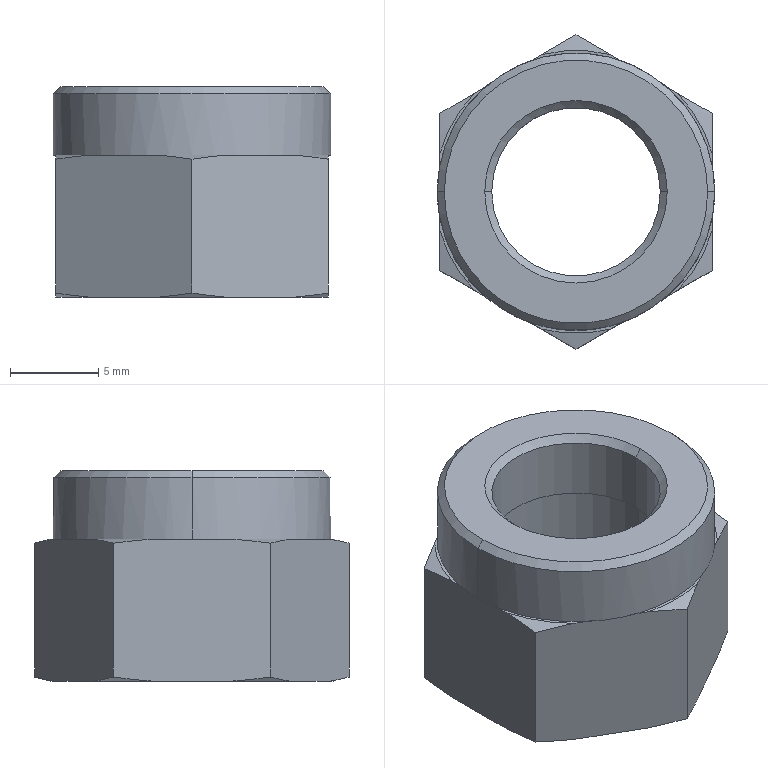Part | SolidWorks | features Cut 3, Boss 1, Chamfer 1, Extrusion 1 | 1 solid | 43 faces | box 15.68 x 17.77 x 11.9 mm | volume 1480 mm3 | plane 21 | cone 16 | cylinder 6 | commonest cylinder face diameters 9.524 x2 10 x2 15.68 x2
STEP:
#1=CARTESIAN_POINT('',(-4.762,0.,11.5));
#2=VERTEX_POINT('',#1);
#3=CARTESIAN_POINT('',(4.762,0.,11.5));
#4=VERTEX_POINT('',#3);
#5=CARTESIAN_POINT('',(0.,0.,11.5));
#6=DIRECTION('',(0.,0.,1.));
#7=DIRECTION('',(1.,0.,0.));
#8=AXIS2_PLACEMENT_3D('',#5,#6,#7);
#9=CIRCLE('',#8,4.762);
#10=EDGE_CURVE('',#2,#4,#9,.T.);
#11=ORIENTED_EDGE('',*,*,#10,.F.);
#12=CARTESIAN_POINT('',(-5.162,0.,11.9));
#13=VERTEX_POINT('',#12);
#14=CARTESIAN_POINT('',(-4.762,0.,11.5));
#15=DIRECTION('',(-0.7071,0.,0.7071));
#16=VECTOR('',#15,1000.);
#17=LINE('',#14,#16);
#18=EDGE_CURVE('',#2,#13,#17,.T.);
#19=ORIENTED_EDGE('',*,*,#18,.T.);
#20=CARTESIAN_POINT('',(5.162,0.,11.9));
#21=VERTEX_POINT('',#20);
#22=CARTESIAN_POINT('',(0.,0.,11.9));
#23=DIRECTION('',(0.,0.,-1.));
#24=DIRECTION('',(1.,0.,0.));
#25=AXIS2_PLACEMENT_3D('',#22,#23,#24);
#26=CIRCLE('',#25,5.162);
#27=EDGE_CURVE('',#21,#13,#26,.T.);
#28=ORIENTED_EDGE('',*,*,#27,.F.);
#29=CARTESIAN_POINT('',(4.762,0.,11.5));
#30=DIRECTION('',(0.7071,0.,0.7071));
#31=VECTOR('',#30,1000.);
#32=LINE('',#29,#31);
#33=EDGE_CURVE('',#4,#21,#32,.T.);
#34=ORIENTED_EDGE('',*,*,#33,.F.);
#35=EDGE_LOOP('',(#11,#19,#28,#34));
#36=FACE_OUTER_BOUND('',#35,.T.);
#37=CARTESIAN_POINT('',(0.,0.,11.5));
#38=DIRECTION('',(0.,0.,1.));
#39=DIRECTION('',(1.,0.,0.));
#40=AXIS2_PLACEMENT_3D('',#37,#38,#39);
#41=CONICAL_SURFACE('',#40,4.762,0.7854);
#42=ADVANCED_FACE('',(#36),#41,.F.);
#43=CARTESIAN_POINT('',(7.44,0.,11.9));
#44=VERTEX_POINT('',#43);
#45=CARTESIAN_POINT('',(-7.44,0.,11.9));
#46=VERTEX_POINT('',#45);
#47=CARTESIAN_POINT('',(0.,0.,11.9));
#48=DIRECTION('',(0.,0.,1.));
#49=DIRECTION('',(1.,0.,0.));
#50=AXIS2_PLACEMENT_3D('',#47,#48,#49);
#51=CIRCLE('',#50,7.44);
#52=EDGE_CURVE('',#44,#46,#51,.T.);
#53=ORIENTED_EDGE('',*,*,#52,.F.);
#54=CARTESIAN_POINT('',(7.84,0.,11.5));
#55=VERTEX_POINT('',#54);
#56=CARTESIAN_POINT('',(7.44,0.,11.9));
#57=DIRECTION('',(0.7071,0.,-0.7071));
#58=VECTOR('',#57,1000.);
#59=LINE('',#56,#58);
#60=EDGE_CURVE('',#44,#55,#59,.T.);
#61=ORIENTED_EDGE('',*,*,#60,.T.);
#62=CARTESIAN_POINT('',(-7.84,0.,11.5));
#63=VERTEX_POINT('',#62);
#64=CARTESIAN_POINT('',(0.,0.,11.5));
#65=DIRECTION('',(0.,0.,-1.));
#66=DIRECTION('',(1.,0.,0.));
#67=AXIS2_PLACEMENT_3D('',#64,#65,#66);
#68=CIRCLE('',#67,7.84);
#69=EDGE_CURVE('',#63,#55,#68,.T.);
#70=ORIENTED_EDGE('',*,*,#69,.F.);
#71=CARTESIAN_POINT('',(-7.44,0.,11.9));
#72=DIRECTION('',(-0.7071,0.,-0.7071));
#73=VECTOR('',#72,1000.);
#74=LINE('',#71,#73);
#75=EDGE_CURVE('',#46,#63,#74,.T.);
#76=ORIENTED_EDGE('',*,*,#75,.F.);
#77=EDGE_LOOP('',(#53,#61,#70,#76));
#78=FACE_OUTER_BOUND('',#77,.T.);
#79=CARTESIAN_POINT('',(0.,0.,11.9));
#80=DIRECTION('',(0.,0.,-1.));
#81=DIRECTION('',(-1.,0.,0.));
#82=AXIS2_PLACEMENT_3D('',#79,#80,#81);
#83=CONICAL_SURFACE('',#82,7.44,0.7854);
#84=ADVANCED_FACE('',(#78),#83,.T.);
#85=CARTESIAN_POINT('',(-4.762,0.,8.04));
#86=VERTEX_POINT('',#85);
#87=CARTESIAN_POINT('',(4.762,0.,8.04));
#88=VERTEX_POINT('',#87);
#89=CARTESIAN_POINT('',(0.,0.,8.04));
#90=DIRECTION('',(0.,0.,1.));
#91=DIRECTION('',(1.,0.,0.));
#92=AXIS2_PLACEMENT_3D('',#89,#90,#91);
#93=CIRCLE('',#92,4.762);
#94=EDGE_CURVE('',#86,#88,#93,.T.);
#95=ORIENTED_EDGE('',*,*,#94,.F.);
#96=CARTESIAN_POINT('',(-4.762,0.,0.));
#97=DIRECTION('',(0.,0.,1.));
#98=VECTOR('',#97,1000.);
#99=LINE('',#96,#98);
#100=EDGE_CURVE('',#86,#2,#99,.T.);
#101=ORIENTED_EDGE('',*,*,#100,.T.);
#102=ORIENTED_EDGE('',*,*,#10,.T.);
#103=CARTESIAN_POINT('',(4.762,0.,0.));
#104=DIRECTION('',(0.,0.,1.));
#105=VECTOR('',#104,1000.);
#106=LINE('',#103,#105);
#107=EDGE_CURVE('',#88,#4,#106,.T.);
#108=ORIENTED_EDGE('',*,*,#107,.F.);
#109=EDGE_LOOP('',(#95,#101,#102,#108));
#110=FACE_OUTER_BOUND('',#109,.T.);
#111=CARTESIAN_POINT('',(0.,0.,0.));
#112=DIRECTION('',(0.,0.,1.));
#113=DIRECTION('',(1.,0.,0.));
#114=AXIS2_PLACEMENT_3D('',#111,#112,#113);
#115=CYLINDRICAL_SURFACE('',#114,4.762);
#116=ADVANCED_FACE('',(#110),#115,.F.);
#117=ORIENTED_EDGE('',*,*,#69,.T.);
#118=CARTESIAN_POINT('',(7.84,0.,8.04));
#119=VERTEX_POINT('',#118);
#120=CARTESIAN_POINT('',(7.84,0.,11.9));
#121=DIRECTION('',(0.,0.,-1.));
#122=VECTOR('',#121,1000.);
#123=LINE('',#120,#122);
#124=EDGE_CURVE('',#55,#119,#123,.T.);
#125=ORIENTED_EDGE('',*,*,#124,.T.);
#126=CARTESIAN_POINT('',(7.695,1.503,8.04));
#127=VERTEX_POINT('',#126);
#128=CARTESIAN_POINT('',(0.,0.,8.04));
#129=DIRECTION('',(0.,0.,1.));
#130=DIRECTION('',(1.,0.,0.));
#131=AXIS2_PLACEMENT_3D('',#128,#129,#130);
#132=CIRCLE('',#131,7.84);
#133=EDGE_CURVE('',#119,#127,#132,.T.);
#134=ORIENTED_EDGE('',*,*,#133,.T.);
#135=CARTESIAN_POINT('',(5.149,5.912,8.04));
#136=VERTEX_POINT('',#135);
#137=CARTESIAN_POINT('',(0.,0.,8.04));
#138=DIRECTION('',(0.,0.,1.));
#139=DIRECTION('',(1.,0.,0.));
#140=AXIS2_PLACEMENT_3D('',#137,#138,#139);
#141=CIRCLE('',#140,7.84);
#142=EDGE_CURVE('',#127,#136,#141,.T.);
#143=ORIENTED_EDGE('',*,*,#142,.T.);
#144=CARTESIAN_POINT('',(2.546,7.415,8.04));
#145=VERTEX_POINT('',#144);
#146=CARTESIAN_POINT('',(0.,0.,8.04));
#147=DIRECTION('',(0.,0.,1.));
#148=DIRECTION('',(1.,0.,0.));
#149=AXIS2_PLACEMENT_3D('',#146,#147,#148);
#150=CIRCLE('',#149,7.84);
#151=EDGE_CURVE('',#136,#145,#150,.T.);
#152=ORIENTED_EDGE('',*,*,#151,.T.);
#153=CARTESIAN_POINT('',(-2.546,7.415,8.04));
#154=VERTEX_POINT('',#153);
#155=CARTESIAN_POINT('',(0.,0.,8.04));
#156=DIRECTION('',(0.,0.,1.));
#157=DIRECTION('',(1.,0.,0.));
#158=AXIS2_PLACEMENT_3D('',#155,#156,#157);
#159=CIRCLE('',#158,7.84);
#160=EDGE_CURVE('',#145,#154,#159,.T.);
#161=ORIENTED_EDGE('',*,*,#160,.T.);
#162=CARTESIAN_POINT('',(-5.149,5.912,8.04));
#163=VERTEX_POINT('',#162);
#164=CARTESIAN_POINT('',(0.,0.,8.04));
#165=DIRECTION('',(0.,0.,1.));
#166=DIRECTION('',(1.,0.,0.));
#167=AXIS2_PLACEMENT_3D('',#164,#165,#166);
#168=CIRCLE('',#167,7.84);
#169=EDGE_CURVE('',#154,#163,#168,.T.);
#170=ORIENTED_EDGE('',*,*,#169,.T.);
#171=CARTESIAN_POINT('',(-7.695,1.503,8.04));
#172=VERTEX_POINT('',#171);
#173=CARTESIAN_POINT('',(0.,0.,8.04));
#174=DIRECTION('',(0.,0.,1.));
#175=DIRECTION('',(1.,0.,0.));
#176=AXIS2_PLACEMENT_3D('',#173,#174,#175);
#177=CIRCLE('',#176,7.84);
#178=EDGE_CURVE('',#163,#172,#177,.T.);
#179=ORIENTED_EDGE('',*,*,#178,.T.);
#180=CARTESIAN_POINT('',(-7.84,0.,8.04));
#181=VERTEX_POINT('',#180);
#182=CARTESIAN_POINT('',(0.,0.,8.04));
#183=DIRECTION('',(0.,0.,1.));
#184=DIRECTION('',(1.,0.,0.));
#185=AXIS2_PLACEMENT_3D('',#182,#183,#184);
#186=CIRCLE('',#185,7.84);
#187=EDGE_CURVE('',#172,#181,#186,.T.);
#188=ORIENTED_EDGE('',*,*,#187,.T.);
#189=CARTESIAN_POINT('',(-7.84,0.,11.9));
#190=DIRECTION('',(0.,0.,-1.));
#191=VECTOR('',#190,1000.);
#192=LINE('',#189,#191);
#193=EDGE_CURVE('',#63,#181,#192,.T.);
#194=ORIENTED_EDGE('',*,*,#193,.F.);
#195=EDGE_LOOP('',(#117,#125,#134,#143,#152,#161,#170,#179,#188,#194));
#196=FACE_OUTER_BOUND('',#195,.T.);
#197=CARTESIAN_POINT('',(0.,0.,11.9));
#198=DIRECTION('',(0.,0.,-1.));
#199=DIRECTION('',(-1.,0.,0.));
#200=AXIS2_PLACEMENT_3D('',#197,#198,#199);
#201=CYLINDRICAL_SURFACE('',#200,7.84);
#202=ADVANCED_FACE('',(#196),#201,.T.);
#203=CARTESIAN_POINT('',(-5.,0.,8.04));
#204=VERTEX_POINT('',#203);
#205=CARTESIAN_POINT('',(5.,0.,8.04));
#206=VERTEX_POINT('',#205);
#207=CARTESIAN_POINT('',(0.,0.,8.04));
#208=DIRECTION('',(0.,0.,1.));
#209=DIRECTION('',(1.,0.,0.));
#210=AXIS2_PLACEMENT_3D('',#207,#208,#209);
#211=CIRCLE('',#210,5.);
#212=EDGE_CURVE('',#204,#206,#211,.T.);
#213=ORIENTED_EDGE('',*,*,#212,.T.);
#214=CARTESIAN_POINT('',(5.,0.,0.));
#215=VERTEX_POINT('',#214);
#216=CARTESIAN_POINT('',(5.,0.,8.04));
#217=DIRECTION('',(0.,0.,-1.));
#218=VECTOR('',#217,1000.);
#219=LINE('',#216,#218);
#220=EDGE_CURVE('',#206,#215,#219,.T.);
#221=ORIENTED_EDGE('',*,*,#220,.T.);
#222=CARTESIAN_POINT('',(-5.,0.,0.));
#223=VERTEX_POINT('',#222);
#224=CARTESIAN_POINT('',(0.,0.,0.));
#225=DIRECTION('',(0.,0.,1.));
#226=DIRECTION('',(1.,0.,0.));
#227=AXIS2_PLACEMENT_3D('',#224,#225,#226);
#228=CIRCLE('',#227,5.);
#229=EDGE_CURVE('',#223,#215,#228,.T.);
#230=ORIENTED_EDGE('',*,*,#229,.F.);
#231=CARTESIAN_POINT('',(-5.,0.,8.04));
#232=DIRECTION('',(0.,0.,-1.));
#233=VECTOR('',#232,1000.);
#234=LINE('',#231,#233);
#235=EDGE_CURVE('',#204,#223,#234,.T.);
#236=ORIENTED_EDGE('',*,*,#235,.F.);
#237=EDGE_LOOP('',(#213,#221,#230,#236));
#238=FACE_OUTER_BOUND('',#237,.T.);
#239=CARTESIAN_POINT('',(0.,0.,8.04));
#240=DIRECTION('',(0.,0.,-1.));
#241=DIRECTION('',(-1.,0.,0.));
#242=AXIS2_PLACEMENT_3D('',#239,#240,#241);
#243=CYLINDRICAL_SURFACE('',#242,5.);
#244=ADVANCED_FACE('',(#238),#243,.F.);
#245=CARTESIAN_POINT('',(7.695,-2.189,8.04));
#246=VERTEX_POINT('',#245);
#247=CARTESIAN_POINT('',(7.695,-1.503,8.04));
#248=VERTEX_POINT('',#247);
#249=CARTESIAN_POINT('',(7.695,-4.442,8.04));
#250=DIRECTION('',(0.,1.,0.));
#251=VECTOR('',#250,1000.);
#252=LINE('',#249,#251);
#253=EDGE_CURVE('',#246,#248,#252,.T.);
#254=ORIENTED_EDGE('',*,*,#253,.T.);
#255=CARTESIAN_POINT('',(5.149,-5.912,8.04));
#256=VERTEX_POINT('',#255);
#257=CARTESIAN_POINT('',(0.,0.,8.04));
#258=DIRECTION('',(0.,0.,1.));
#259=DIRECTION('',(1.,0.,0.));
#260=AXIS2_PLACEMENT_3D('',#257,#258,#259);
#261=CIRCLE('',#260,7.84);
#262=EDGE_CURVE('',#256,#248,#261,.T.);
#263=ORIENTED_EDGE('',*,*,#262,.F.);
#264=CARTESIAN_POINT('',(5.743,-5.569,8.04));
#265=VERTEX_POINT('',#264);
#266=CARTESIAN_POINT('',(0.,-8.885,8.04));
#267=DIRECTION('',(0.866,0.5,0.));
#268=VECTOR('',#267,1000.);
#269=LINE('',#266,#268);
#270=EDGE_CURVE('',#256,#265,#269,.T.);
#271=ORIENTED_EDGE('',*,*,#270,.T.);
#272=CARTESIAN_POINT('',(0.,0.,8.04));
#273=DIRECTION('',(0.,0.,1.));
#274=DIRECTION('',(1.,0.,0.));
#275=AXIS2_PLACEMENT_3D('',#272,#273,#274);
#276=CIRCLE('',#275,8.);
#277=EDGE_CURVE('',#265,#246,#276,.T.);
#278=ORIENTED_EDGE('',*,*,#277,.T.);
#279=EDGE_LOOP('',(#254,#263,#271,#278));
#280=FACE_OUTER_BOUND('',#279,.T.);
#281=CARTESIAN_POINT('',(-7.695,13.328,8.04));
#282=DIRECTION('',(0.,0.,1.));
#283=DIRECTION('',(1.,0.,0.));
#284=AXIS2_PLACEMENT_3D('',#281,#282,#283);
#285=PLANE('',#284);
#286=ADVANCED_FACE('',(#280),#285,.T.);
#287=CARTESIAN_POINT('',(1.951,-7.758,8.04));
#288=VERTEX_POINT('',#287);
#289=CARTESIAN_POINT('',(2.546,-7.415,8.04));
#290=VERTEX_POINT('',#289);
#291=CARTESIAN_POINT('',(0.,-8.885,8.04));
#292=DIRECTION('',(0.866,0.5,0.));
#293=VECTOR('',#292,1000.);
#294=LINE('',#291,#293);
#295=EDGE_CURVE('',#288,#290,#294,.T.);
#296=ORIENTED_EDGE('',*,*,#295,.T.);
#297=CARTESIAN_POINT('',(-2.546,-7.415,8.04));
#298=VERTEX_POINT('',#297);
#299=CARTESIAN_POINT('',(0.,0.,8.04));
#300=DIRECTION('',(0.,0.,1.));
#301=DIRECTION('',(1.,0.,0.));
#302=AXIS2_PLACEMENT_3D('',#299,#300,#301);
#303=CIRCLE('',#302,7.84);
#304=EDGE_CURVE('',#298,#290,#303,.T.);
#305=ORIENTED_EDGE('',*,*,#304,.F.);
#306=CARTESIAN_POINT('',(-1.951,-7.758,8.04));
#307=VERTEX_POINT('',#306);
#308=CARTESIAN_POINT('',(-7.695,-4.442,8.04));
#309=DIRECTION('',(0.866,-0.5,0.));
#310=VECTOR('',#309,1000.);
#311=LINE('',#308,#310);
#312=EDGE_CURVE('',#298,#307,#311,.T.);
#313=ORIENTED_EDGE('',*,*,#312,.T.);
#314=CARTESIAN_POINT('',(0.,0.,8.04));
#315=DIRECTION('',(0.,0.,1.));
#316=DIRECTION('',(1.,0.,0.));
#317=AXIS2_PLACEMENT_3D('',#314,#315,#316);
#318=CIRCLE('',#317,8.);
#319=EDGE_CURVE('',#307,#288,#318,.T.);
#320=ORIENTED_EDGE('',*,*,#319,.T.);
#321=EDGE_LOOP('',(#296,#305,#313,#320));
#322=FACE_OUTER_BOUND('',#321,.T.);
#323=CARTESIAN_POINT('',(-7.695,13.328,8.04));
#324=DIRECTION('',(0.,0.,1.));
#325=DIRECTION('',(1.,0.,0.));
#326=AXIS2_PLACEMENT_3D('',#323,#324,#325);
#327=PLANE('',#326);
#328=ADVANCED_FACE('',(#322),#327,.T.);
#329=CARTESIAN_POINT('',(-5.743,-5.569,8.04));
#330=VERTEX_POINT('',#329);
#331=CARTESIAN_POINT('',(-5.149,-5.912,8.04));
#332=VERTEX_POINT('',#331);
#333=CARTESIAN_POINT('',(-7.695,-4.442,8.04));
#334=DIRECTION('',(0.866,-0.5,0.));
#335=VECTOR('',#334,1000.);
#336=LINE('',#333,#335);
#337=EDGE_CURVE('',#330,#332,#336,.T.);
#338=ORIENTED_EDGE('',*,*,#337,.T.);
#339=CARTESIAN_POINT('',(-7.695,-1.503,8.04));
#340=VERTEX_POINT('',#339);
#341=CARTESIAN_POINT('',(0.,0.,8.04));
#342=DIRECTION('',(0.,0.,1.));
#343=DIRECTION('',(1.,0.,0.));
#344=AXIS2_PLACEMENT_3D('',#341,#342,#343);
#345=CIRCLE('',#344,7.84);
#346=EDGE_CURVE('',#340,#332,#345,.T.);
#347=ORIENTED_EDGE('',*,*,#346,.F.);
#348=CARTESIAN_POINT('',(-7.695,-2.189,8.04));
#349=VERTEX_POINT('',#348);
#350=CARTESIAN_POINT('',(-7.695,4.443,8.04));
#351=DIRECTION('',(0.,-1.,0.));
#352=VECTOR('',#351,1000.);
#353=LINE('',#350,#352);
#354=EDGE_CURVE('',#340,#349,#353,.T.);
#355=ORIENTED_EDGE('',*,*,#354,.T.);
#356=CARTESIAN_POINT('',(0.,0.,8.04));
#357=DIRECTION('',(0.,0.,1.));
#358=DIRECTION('',(1.,0.,0.));
#359=AXIS2_PLACEMENT_3D('',#356,#357,#358);
#360=CIRCLE('',#359,8.);
#361=EDGE_CURVE('',#349,#330,#360,.T.);
#362=ORIENTED_EDGE('',*,*,#361,.T.);
#363=EDGE_LOOP('',(#338,#347,#355,#362));
#364=FACE_OUTER_BOUND('',#363,.T.);
#365=CARTESIAN_POINT('',(-7.695,13.328,8.04));
#366=DIRECTION('',(0.,0.,1.));
#367=DIRECTION('',(1.,0.,0.));
#368=AXIS2_PLACEMENT_3D('',#365,#366,#367);
#369=PLANE('',#368);
#370=ADVANCED_FACE('',(#364),#369,.T.);
#371=CARTESIAN_POINT('',(-7.695,2.189,8.04));
#372=VERTEX_POINT('',#371);
#373=CARTESIAN_POINT('',(-7.695,4.443,8.04));
#374=DIRECTION('',(0.,-1.,0.));
#375=VECTOR('',#374,1000.);
#376=LINE('',#373,#375);
#377=EDGE_CURVE('',#372,#172,#376,.T.);
#378=ORIENTED_EDGE('',*,*,#377,.T.);
#379=ORIENTED_EDGE('',*,*,#178,.F.);
#380=CARTESIAN_POINT('',(-5.743,5.569,8.04));
#381=VERTEX_POINT('',#380);
#382=CARTESIAN_POINT('',(0.,8.885,8.04));
#383=DIRECTION('',(-0.866,-0.5,0.));
#384=VECTOR('',#383,1000.);
#385=LINE('',#382,#384);
#386=EDGE_CURVE('',#163,#381,#385,.T.);
#387=ORIENTED_EDGE('',*,*,#386,.T.);
#388=CARTESIAN_POINT('',(0.,0.,8.04));
#389=DIRECTION('',(0.,0.,1.));
#390=DIRECTION('',(1.,0.,0.));
#391=AXIS2_PLACEMENT_3D('',#388,#389,#390);
#392=CIRCLE('',#391,8.);
#393=EDGE_CURVE('',#381,#372,#392,.T.);
#394=ORIENTED_EDGE('',*,*,#393,.T.);
#395=EDGE_LOOP('',(#378,#379,#387,#394));
#396=FACE_OUTER_BOUND('',#395,.T.);
#397=CARTESIAN_POINT('',(-7.695,13.328,8.04));
#398=DIRECTION('',(0.,0.,1.));
#399=DIRECTION('',(1.,0.,0.));
#400=AXIS2_PLACEMENT_3D('',#397,#398,#399);
#401=PLANE('',#400);
#402=ADVANCED_FACE('',(#396),#401,.T.);
#403=CARTESIAN_POINT('',(-1.951,7.758,8.04));
#404=VERTEX_POINT('',#403);
#405=CARTESIAN_POINT('',(0.,8.885,8.04));
#406=DIRECTION('',(-0.866,-0.5,0.));
#407=VECTOR('',#406,1000.);
#408=LINE('',#405,#407);
#409=EDGE_CURVE('',#404,#154,#408,.T.);
#410=ORIENTED_EDGE('',*,*,#409,.T.);
#411=ORIENTED_EDGE('',*,*,#160,.F.);
#412=CARTESIAN_POINT('',(1.951,7.758,8.04));
#413=VERTEX_POINT('',#412);
#414=CARTESIAN_POINT('',(7.695,4.443,8.04));
#415=DIRECTION('',(-0.866,0.5,0.));
#416=VECTOR('',#415,1000.);
#417=LINE('',#414,#416);
#418=EDGE_CURVE('',#145,#413,#417,.T.);
#419=ORIENTED_EDGE('',*,*,#418,.T.);
#420=CARTESIAN_POINT('',(0.,0.,8.04));
#421=DIRECTION('',(0.,0.,1.));
#422=DIRECTION('',(1.,0.,0.));
#423=AXIS2_PLACEMENT_3D('',#420,#421,#422);
#424=CIRCLE('',#423,8.);
#425=EDGE_CURVE('',#413,#404,#424,.T.);
#426=ORIENTED_EDGE('',*,*,#425,.T.);
#427=EDGE_LOOP('',(#410,#411,#419,#426));
#428=FACE_OUTER_BOUND('',#427,.T.);
#429=CARTESIAN_POINT('',(-7.695,13.328,8.04));
#430=DIRECTION('',(0.,0.,1.));
#431=DIRECTION('',(1.,0.,0.));
#432=AXIS2_PLACEMENT_3D('',#429,#430,#431);
#433=PLANE('',#432);
#434=ADVANCED_FACE('',(#428),#433,.T.);
#435=CARTESIAN_POINT('',(5.743,5.569,8.04));
#436=VERTEX_POINT('',#435);
#437=CARTESIAN_POINT('',(7.695,4.443,8.04));
#438=DIRECTION('',(-0.866,0.5,0.));
#439=VECTOR('',#438,1000.);
#440=LINE('',#437,#439);
#441=EDGE_CURVE('',#436,#136,#440,.T.);
#442=ORIENTED_EDGE('',*,*,#441,.T.);
#443=ORIENTED_EDGE('',*,*,#142,.F.);
#444=CARTESIAN_POINT('',(7.695,2.189,8.04));
#445=VERTEX_POINT('',#444);
#446=CARTESIAN_POINT('',(7.695,-4.442,8.04));
#447=DIRECTION('',(0.,1.,0.));
#448=VECTOR('',#447,1000.);
#449=LINE('',#446,#448);
#450=EDGE_CURVE('',#127,#445,#449,.T.);
#451=ORIENTED_EDGE('',*,*,#450,.T.);
#452=CARTESIAN_POINT('',(0.,0.,8.04));
#453=DIRECTION('',(0.,0.,1.));
#454=DIRECTION('',(1.,0.,0.));
#455=AXIS2_PLACEMENT_3D('',#452,#453,#454);
#456=CIRCLE('',#455,8.);
#457=EDGE_CURVE('',#445,#436,#456,.T.);
#458=ORIENTED_EDGE('',*,*,#457,.T.);
#459=EDGE_LOOP('',(#442,#443,#451,#458));
#460=FACE_OUTER_BOUND('',#459,.T.);
#461=CARTESIAN_POINT('',(-7.695,13.328,8.04));
#462=DIRECTION('',(0.,0.,1.));
#463=DIRECTION('',(1.,0.,0.));
#464=AXIS2_PLACEMENT_3D('',#461,#462,#463);
#465=PLANE('',#464);
#466=ADVANCED_FACE('',(#460),#465,.T.);
#467=CARTESIAN_POINT('',(0.,8.885,0.2371));
#468=VERTEX_POINT('',#467);
#469=CARTESIAN_POINT('',(1.951,7.758,0.));
#470=VERTEX_POINT('',#469);
#471=CARTESIAN_POINT('',(0.,8.885,0.2371));
#472=CARTESIAN_POINT('',(0.6483,8.511,0.1368));
#473=CARTESIAN_POINT('',(1.298,8.135,0.05528));
#474=CARTESIAN_POINT('',(1.951,7.758,0.));
#475=B_SPLINE_CURVE_WITH_KNOTS('',3,(#471,#472,#473,#474),.UNSPECIFIED.,.F.,.F.,(4,4),(0.008381,0.01065),.UNSPECIFIED.);
#476=EDGE_CURVE('',#468,#470,#475,.T.);
#477=ORIENTED_EDGE('',*,*,#476,.F.);
#478=CARTESIAN_POINT('',(0.,8.885,7.803));
#479=VERTEX_POINT('',#478);
#480=CARTESIAN_POINT('',(0.,8.885,8.04));
#481=DIRECTION('',(0.,0.,-1.));
#482=VECTOR('',#481,1000.);
#483=LINE('',#480,#482);
#484=EDGE_CURVE('',#479,#468,#483,.T.);
#485=ORIENTED_EDGE('',*,*,#484,.F.);
#486=CARTESIAN_POINT('',(1.951,7.758,8.04));
#487=CARTESIAN_POINT('',(1.298,8.135,7.985));
#488=CARTESIAN_POINT('',(0.6473,8.511,7.903));
#489=CARTESIAN_POINT('',(0.,8.885,7.803));
#490=B_SPLINE_CURVE_WITH_KNOTS('',3,(#486,#487,#488,#489),.UNSPECIFIED.,.F.,.F.,(4,4),(0.01499,0.01722),.UNSPECIFIED.);
#491=EDGE_CURVE('',#413,#479,#490,.T.);
#492=ORIENTED_EDGE('',*,*,#491,.F.);
#493=ORIENTED_EDGE('',*,*,#418,.F.);
#494=CARTESIAN_POINT('',(7.695,4.443,8.04));
#495=DIRECTION('',(-0.866,0.5,0.));
#496=VECTOR('',#495,1000.);
#497=LINE('',#494,#496);
#498=EDGE_CURVE('',#136,#145,#497,.T.);
#499=ORIENTED_EDGE('',*,*,#498,.F.);
#500=ORIENTED_EDGE('',*,*,#441,.F.);
#501=CARTESIAN_POINT('',(7.695,4.443,7.803));
#502=VERTEX_POINT('',#501);
#503=CARTESIAN_POINT('',(7.695,4.443,7.803));
#504=CARTESIAN_POINT('',(7.046,4.817,7.903));
#505=CARTESIAN_POINT('',(6.396,5.192,7.985));
#506=CARTESIAN_POINT('',(5.743,5.569,8.04));
#507=B_SPLINE_CURVE_WITH_KNOTS('',3,(#503,#504,#505,#506),.UNSPECIFIED.,.F.,.F.,(4,4),(0.008381,0.01065),.UNSPECIFIED.);
#508=EDGE_CURVE('',#502,#436,#507,.T.);
#509=ORIENTED_EDGE('',*,*,#508,.F.);
#510=CARTESIAN_POINT('',(7.695,4.443,0.2371));
#511=VERTEX_POINT('',#510);
#512=CARTESIAN_POINT('',(7.695,4.443,8.04));
#513=DIRECTION('',(0.,0.,-1.));
#514=VECTOR('',#513,1000.);
#515=LINE('',#512,#514);
#516=EDGE_CURVE('',#502,#511,#515,.T.);
#517=ORIENTED_EDGE('',*,*,#516,.T.);
#518=CARTESIAN_POINT('',(5.743,5.569,0.));
#519=VERTEX_POINT('',#518);
#520=CARTESIAN_POINT('',(5.743,5.569,0.));
#521=CARTESIAN_POINT('',(6.396,5.192,0.05529));
#522=CARTESIAN_POINT('',(7.047,4.816,0.137));
#523=CARTESIAN_POINT('',(7.695,4.443,0.2371));
#524=B_SPLINE_CURVE_WITH_KNOTS('',3,(#520,#521,#522,#523),.UNSPECIFIED.,.F.,.F.,(4,4),(0.01499,0.01722),.UNSPECIFIED.);
#525=EDGE_CURVE('',#519,#511,#524,.T.);
#526=ORIENTED_EDGE('',*,*,#525,.F.);
#527=CARTESIAN_POINT('',(7.695,4.443,0.));
#528=DIRECTION('',(-0.866,0.5,0.));
#529=VECTOR('',#528,1000.);
#530=LINE('',#527,#529);
#531=EDGE_CURVE('',#519,#470,#530,.T.);
#532=ORIENTED_EDGE('',*,*,#531,.T.);
#533=EDGE_LOOP('',(#477,#485,#492,#493,#499,#500,#509,#517,#526,#532));
#534=FACE_OUTER_BOUND('',#533,.T.);
#535=CARTESIAN_POINT('',(7.695,4.443,8.04));
#536=DIRECTION('',(-0.5,-0.866,0.));
#537=DIRECTION('',(0.866,-0.5,0.));
#538=AXIS2_PLACEMENT_3D('',#535,#536,#537);
#539=PLANE('',#538);
#540=ADVANCED_FACE('',(#534),#539,.F.);
#541=CARTESIAN_POINT('',(-7.695,4.443,0.2371));
#542=VERTEX_POINT('',#541);
#543=CARTESIAN_POINT('',(-5.743,5.569,0.));
#544=VERTEX_POINT('',#543);
#545=CARTESIAN_POINT('',(-7.695,4.443,0.2371));
#546=CARTESIAN_POINT('',(-7.046,4.817,0.1368));
#547=CARTESIAN_POINT('',(-6.396,5.192,0.05528));
#548=CARTESIAN_POINT('',(-5.743,5.569,0.));
#549=B_SPLINE_CURVE_WITH_KNOTS('',3,(#545,#546,#547,#548),.UNSPECIFIED.,.F.,.F.,(4,4),(0.008381,0.01065),.UNSPECIFIED.);
#550=EDGE_CURVE('',#542,#544,#549,.T.);
#551=ORIENTED_EDGE('',*,*,#550,.F.);
#552=CARTESIAN_POINT('',(-7.695,4.443,7.803));
#553=VERTEX_POINT('',#552);
#554=CARTESIAN_POINT('',(-7.695,4.443,8.04));
#555=DIRECTION('',(0.,0.,-1.));
#556=VECTOR('',#555,1000.);
#557=LINE('',#554,#556);
#558=EDGE_CURVE('',#553,#542,#557,.T.);
#559=ORIENTED_EDGE('',*,*,#558,.F.);
#560=CARTESIAN_POINT('',(-5.743,5.569,8.04));
#561=CARTESIAN_POINT('',(-6.396,5.192,7.985));
#562=CARTESIAN_POINT('',(-7.047,4.816,7.903));
#563=CARTESIAN_POINT('',(-7.695,4.443,7.803));
#564=B_SPLINE_CURVE_WITH_KNOTS('',3,(#560,#561,#562,#563),.UNSPECIFIED.,.F.,.F.,(4,4),(0.01499,0.01722),.UNSPECIFIED.);
#565=EDGE_CURVE('',#381,#553,#564,.T.);
#566=ORIENTED_EDGE('',*,*,#565,.F.);
#567=ORIENTED_EDGE('',*,*,#386,.F.);
#568=CARTESIAN_POINT('',(0.,8.885,8.04));
#569=DIRECTION('',(-0.866,-0.5,0.));
#570=VECTOR('',#569,1000.);
#571=LINE('',#568,#570);
#572=EDGE_CURVE('',#154,#163,#571,.T.);
#573=ORIENTED_EDGE('',*,*,#572,.F.);
#574=ORIENTED_EDGE('',*,*,#409,.F.);
#575=CARTESIAN_POINT('',(0.,8.885,7.803));
#576=CARTESIAN_POINT('',(-0.6483,8.511,7.903));
#577=CARTESIAN_POINT('',(-1.298,8.135,7.985));
#578=CARTESIAN_POINT('',(-1.951,7.758,8.04));
#579=B_SPLINE_CURVE_WITH_KNOTS('',3,(#575,#576,#577,#578),.UNSPECIFIED.,.F.,.F.,(4,4),(0.008381,0.01065),.UNSPECIFIED.);
#580=EDGE_CURVE('',#479,#404,#579,.T.);
#581=ORIENTED_EDGE('',*,*,#580,.F.);
#582=ORIENTED_EDGE('',*,*,#484,.T.);
#583=CARTESIAN_POINT('',(-1.951,7.758,0.));
#584=VERTEX_POINT('',#583);
#585=CARTESIAN_POINT('',(-1.951,7.758,0.));
#586=CARTESIAN_POINT('',(-1.298,8.135,0.05529));
#587=CARTESIAN_POINT('',(-0.6473,8.511,0.137));
#588=CARTESIAN_POINT('',(0.,8.885,0.2371));
#589=B_SPLINE_CURVE_WITH_KNOTS('',3,(#585,#586,#587,#588),.UNSPECIFIED.,.F.,.F.,(4,4),(0.01499,0.01722),.UNSPECIFIED.);
#590=EDGE_CURVE('',#584,#468,#589,.T.);
#591=ORIENTED_EDGE('',*,*,#590,.F.);
#592=CARTESIAN_POINT('',(0.,8.885,0.));
#593=DIRECTION('',(-0.866,-0.5,0.));
#594=VECTOR('',#593,1000.);
#595=LINE('',#592,#594);
#596=EDGE_CURVE('',#584,#544,#595,.T.);
#597=ORIENTED_EDGE('',*,*,#596,.T.);
#598=EDGE_LOOP('',(#551,#559,#566,#567,#573,#574,#581,#582,#591,#597));
#599=FACE_OUTER_BOUND('',#598,.T.);
#600=CARTESIAN_POINT('',(0.,8.885,8.04));
#601=DIRECTION('',(0.5,-0.866,0.));
#602=DIRECTION('',(0.866,0.5,0.));
#603=AXIS2_PLACEMENT_3D('',#600,#601,#602);
#604=PLANE('',#603);
#605=ADVANCED_FACE('',(#599),#604,.F.);
#606=CARTESIAN_POINT('',(-7.695,-4.442,0.2371));
#607=VERTEX_POINT('',#606);
#608=CARTESIAN_POINT('',(-7.695,-2.189,0.));
#609=VERTEX_POINT('',#608);
#610=CARTESIAN_POINT('',(-7.695,-4.442,0.2371));
#611=CARTESIAN_POINT('',(-7.695,-3.694,0.1368));
#612=CARTESIAN_POINT('',(-7.695,-2.943,0.05527));
#613=CARTESIAN_POINT('',(-7.695,-2.189,0.));
#614=B_SPLINE_CURVE_WITH_KNOTS('',3,(#610,#611,#612,#613),.UNSPECIFIED.,.F.,.F.,(4,4),(0.007248,0.009514),.UNSPECIFIED.);
#615=EDGE_CURVE('',#607,#609,#614,.T.);
#616=ORIENTED_EDGE('',*,*,#615,.F.);
#617=CARTESIAN_POINT('',(-7.695,-4.442,7.803));
#618=VERTEX_POINT('',#617);
#619=CARTESIAN_POINT('',(-7.695,-4.442,8.04));
#620=DIRECTION('',(0.,0.,-1.));
#621=VECTOR('',#620,1000.);
#622=LINE('',#619,#621);
#623=EDGE_CURVE('',#618,#607,#622,.T.);
#624=ORIENTED_EDGE('',*,*,#623,.F.);
#625=CARTESIAN_POINT('',(-7.695,-2.189,8.04));
#626=CARTESIAN_POINT('',(-7.695,-2.942,7.985));
#627=CARTESIAN_POINT('',(-7.695,-3.695,7.903));
#628=CARTESIAN_POINT('',(-7.695,-4.442,7.803));
#629=B_SPLINE_CURVE_WITH_KNOTS('',3,(#625,#626,#627,#628),.UNSPECIFIED.,.F.,.F.,(4,4),(0.01387,0.01609),.UNSPECIFIED.);
#630=EDGE_CURVE('',#349,#618,#629,.T.);
#631=ORIENTED_EDGE('',*,*,#630,.F.);
#632=ORIENTED_EDGE('',*,*,#354,.F.);
#633=CARTESIAN_POINT('',(-7.695,4.443,8.04));
#634=DIRECTION('',(0.,-1.,0.));
#635=VECTOR('',#634,1000.);
#636=LINE('',#633,#635);
#637=EDGE_CURVE('',#172,#340,#636,.T.);
#638=ORIENTED_EDGE('',*,*,#637,.F.);
#639=ORIENTED_EDGE('',*,*,#377,.F.);
#640=CARTESIAN_POINT('',(-7.695,4.443,7.803));
#641=CARTESIAN_POINT('',(-7.695,3.694,7.903));
#642=CARTESIAN_POINT('',(-7.695,2.943,7.985));
#643=CARTESIAN_POINT('',(-7.695,2.189,8.04));
#644=B_SPLINE_CURVE_WITH_KNOTS('',3,(#640,#641,#642,#643),.UNSPECIFIED.,.F.,.F.,(4,4),(0.007248,0.009514),.UNSPECIFIED.);
#645=EDGE_CURVE('',#553,#372,#644,.T.);
#646=ORIENTED_EDGE('',*,*,#645,.F.);
#647=ORIENTED_EDGE('',*,*,#558,.T.);
#648=CARTESIAN_POINT('',(-7.695,2.189,0.));
#649=VERTEX_POINT('',#648);
#650=CARTESIAN_POINT('',(-7.695,2.189,0.));
#651=CARTESIAN_POINT('',(-7.695,2.942,0.05521));
#652=CARTESIAN_POINT('',(-7.695,3.695,0.137));
#653=CARTESIAN_POINT('',(-7.695,4.443,0.2371));
#654=B_SPLINE_CURVE_WITH_KNOTS('',3,(#650,#651,#652,#653),.UNSPECIFIED.,.F.,.F.,(4,4),(0.01387,0.01609),.UNSPECIFIED.);
#655=EDGE_CURVE('',#649,#542,#654,.T.);
#656=ORIENTED_EDGE('',*,*,#655,.F.);
#657=CARTESIAN_POINT('',(-7.695,4.443,0.));
#658=DIRECTION('',(0.,-1.,0.));
#659=VECTOR('',#658,1000.);
#660=LINE('',#657,#659);
#661=EDGE_CURVE('',#649,#609,#660,.T.);
#662=ORIENTED_EDGE('',*,*,#661,.T.);
#663=EDGE_LOOP('',(#616,#624,#631,#632,#638,#639,#646,#647,#656,#662));
#664=FACE_OUTER_BOUND('',#663,.T.);
#665=CARTESIAN_POINT('',(-7.695,4.443,8.04));
#666=DIRECTION('',(1.,0.,0.));
#667=DIRECTION('',(0.,0.,-1.));
#668=AXIS2_PLACEMENT_3D('',#665,#666,#667);
#669=PLANE('',#668);
#670=ADVANCED_FACE('',(#664),#669,.F.);
#671=CARTESIAN_POINT('',(0.,-8.885,0.2371));
#672=VERTEX_POINT('',#671);
#673=CARTESIAN_POINT('',(-1.951,-7.758,0.));
#674=VERTEX_POINT('',#673);
#675=CARTESIAN_POINT('',(0.,-8.885,0.2371));
#676=CARTESIAN_POINT('',(-0.6483,-8.511,0.1368));
#677=CARTESIAN_POINT('',(-1.298,-8.135,0.05528));
#678=CARTESIAN_POINT('',(-1.951,-7.758,0.));
#679=B_SPLINE_CURVE_WITH_KNOTS('',3,(#675,#676,#677,#678),.UNSPECIFIED.,.F.,.F.,(4,4),(0.008381,0.01065),.UNSPECIFIED.);
#680=EDGE_CURVE('',#672,#674,#679,.T.);
#681=ORIENTED_EDGE('',*,*,#680,.F.);
#682=CARTESIAN_POINT('',(0.,-8.885,7.803));
#683=VERTEX_POINT('',#682);
#684=CARTESIAN_POINT('',(0.,-8.885,8.04));
#685=DIRECTION('',(0.,0.,-1.));
#686=VECTOR('',#685,1000.);
#687=LINE('',#684,#686);
#688=EDGE_CURVE('',#683,#672,#687,.T.);
#689=ORIENTED_EDGE('',*,*,#688,.F.);
#690=CARTESIAN_POINT('',(-1.951,-7.758,8.04));
#691=CARTESIAN_POINT('',(-1.298,-8.135,7.985));
#692=CARTESIAN_POINT('',(-0.6473,-8.511,7.903));
#693=CARTESIAN_POINT('',(0.,-8.885,7.803));
#694=B_SPLINE_CURVE_WITH_KNOTS('',3,(#690,#691,#692,#693),.UNSPECIFIED.,.F.,.F.,(4,4),(0.01499,0.01722),.UNSPECIFIED.);
#695=EDGE_CURVE('',#307,#683,#694,.T.);
#696=ORIENTED_EDGE('',*,*,#695,.F.);
#697=ORIENTED_EDGE('',*,*,#312,.F.);
#698=CARTESIAN_POINT('',(-7.695,-4.442,8.04));
#699=DIRECTION('',(0.866,-0.5,0.));
#700=VECTOR('',#699,1000.);
#701=LINE('',#698,#700);
#702=EDGE_CURVE('',#332,#298,#701,.T.);
#703=ORIENTED_EDGE('',*,*,#702,.F.);
#704=ORIENTED_EDGE('',*,*,#337,.F.);
#705=CARTESIAN_POINT('',(-7.695,-4.442,7.803));
#706=CARTESIAN_POINT('',(-7.046,-4.817,7.903));
#707=CARTESIAN_POINT('',(-6.396,-5.192,7.985));
#708=CARTESIAN_POINT('',(-5.743,-5.569,8.04));
#709=B_SPLINE_CURVE_WITH_KNOTS('',3,(#705,#706,#707,#708),.UNSPECIFIED.,.F.,.F.,(4,4),(0.008381,0.01065),.UNSPECIFIED.);
#710=EDGE_CURVE('',#618,#330,#709,.T.);
#711=ORIENTED_EDGE('',*,*,#710,.F.);
#712=ORIENTED_EDGE('',*,*,#623,.T.);
#713=CARTESIAN_POINT('',(-5.743,-5.569,0.));
#714=VERTEX_POINT('',#713);
#715=CARTESIAN_POINT('',(-5.743,-5.569,0.));
#716=CARTESIAN_POINT('',(-6.396,-5.192,0.05529));
#717=CARTESIAN_POINT('',(-7.047,-4.816,0.137));
#718=CARTESIAN_POINT('',(-7.695,-4.442,0.2371));
#719=B_SPLINE_CURVE_WITH_KNOTS('',3,(#715,#716,#717,#718),.UNSPECIFIED.,.F.,.F.,(4,4),(0.01499,0.01722),.UNSPECIFIED.);
#720=EDGE_CURVE('',#714,#607,#719,.T.);
#721=ORIENTED_EDGE('',*,*,#720,.F.);
#722=CARTESIAN_POINT('',(-7.695,-4.442,0.));
#723=DIRECTION('',(0.866,-0.5,0.));
#724=VECTOR('',#723,1000.);
#725=LINE('',#722,#724);
#726=EDGE_CURVE('',#714,#674,#725,.T.);
#727=ORIENTED_EDGE('',*,*,#726,.T.);
#728=EDGE_LOOP('',(#681,#689,#696,#697,#703,#704,#711,#712,#721,#727));
#729=FACE_OUTER_BOUND('',#728,.T.);
#730=CARTESIAN_POINT('',(-7.695,-4.442,8.04));
#731=DIRECTION('',(0.5,0.866,0.));
#732=DIRECTION('',(-0.866,0.5,0.));
#733=AXIS2_PLACEMENT_3D('',#730,#731,#732);
#734=PLANE('',#733);
#735=ADVANCED_FACE('',(#729),#734,.F.);
#736=CARTESIAN_POINT('',(7.695,-4.443,0.2371));
#737=VERTEX_POINT('',#736);
#738=CARTESIAN_POINT('',(5.743,-5.569,0.));
#739=VERTEX_POINT('',#738);
#740=CARTESIAN_POINT('',(7.695,-4.443,0.2371));
#741=CARTESIAN_POINT('',(7.046,-4.817,0.1368));
#742=CARTESIAN_POINT('',(6.396,-5.192,0.05528));
#743=CARTESIAN_POINT('',(5.743,-5.569,0.));
#744=B_SPLINE_CURVE_WITH_KNOTS('',3,(#740,#741,#742,#743),.UNSPECIFIED.,.F.,.F.,(4,4),(0.008381,0.01065),.UNSPECIFIED.);
#745=EDGE_CURVE('',#737,#739,#744,.T.);
#746=ORIENTED_EDGE('',*,*,#745,.F.);
#747=CARTESIAN_POINT('',(7.695,-4.442,7.803));
#748=VERTEX_POINT('',#747);
#749=CARTESIAN_POINT('',(7.695,-4.442,8.04));
#750=DIRECTION('',(0.,0.,-1.));
#751=VECTOR('',#750,1000.);
#752=LINE('',#749,#751);
#753=EDGE_CURVE('',#748,#737,#752,.T.);
#754=ORIENTED_EDGE('',*,*,#753,.F.);
#755=CARTESIAN_POINT('',(5.743,-5.569,8.04));
#756=CARTESIAN_POINT('',(6.396,-5.192,7.985));
#757=CARTESIAN_POINT('',(7.047,-4.816,7.903));
#758=CARTESIAN_POINT('',(7.695,-4.442,7.803));
#759=B_SPLINE_CURVE_WITH_KNOTS('',3,(#755,#756,#757,#758),.UNSPECIFIED.,.F.,.F.,(4,4),(0.01499,0.01722),.UNSPECIFIED.);
#760=EDGE_CURVE('',#265,#748,#759,.T.);
#761=ORIENTED_EDGE('',*,*,#760,.F.);
#762=ORIENTED_EDGE('',*,*,#270,.F.);
#763=CARTESIAN_POINT('',(0.,-8.885,8.04));
#764=DIRECTION('',(0.866,0.5,0.));
#765=VECTOR('',#764,1000.);
#766=LINE('',#763,#765);
#767=EDGE_CURVE('',#290,#256,#766,.T.);
#768=ORIENTED_EDGE('',*,*,#767,.F.);
#769=ORIENTED_EDGE('',*,*,#295,.F.);
#770=CARTESIAN_POINT('',(0.,-8.885,7.803));
#771=CARTESIAN_POINT('',(0.6483,-8.511,7.903));
#772=CARTESIAN_POINT('',(1.298,-8.135,7.985));
#773=CARTESIAN_POINT('',(1.951,-7.758,8.04));
#774=B_SPLINE_CURVE_WITH_KNOTS('',3,(#770,#771,#772,#773),.UNSPECIFIED.,.F.,.F.,(4,4),(0.008381,0.01065),.UNSPECIFIED.);
#775=EDGE_CURVE('',#683,#288,#774,.T.);
#776=ORIENTED_EDGE('',*,*,#775,.F.);
#777=ORIENTED_EDGE('',*,*,#688,.T.);
#778=CARTESIAN_POINT('',(1.951,-7.758,0.));
#779=VERTEX_POINT('',#778);
#780=CARTESIAN_POINT('',(1.951,-7.758,0.));
#781=CARTESIAN_POINT('',(1.298,-8.135,0.05529));
#782=CARTESIAN_POINT('',(0.6473,-8.511,0.137));
#783=CARTESIAN_POINT('',(0.,-8.885,0.2371));
#784=B_SPLINE_CURVE_WITH_KNOTS('',3,(#780,#781,#782,#783),.UNSPECIFIED.,.F.,.F.,(4,4),(0.01499,0.01722),.UNSPECIFIED.);
#785=EDGE_CURVE('',#779,#672,#784,.T.);
#786=ORIENTED_EDGE('',*,*,#785,.F.);
#787=CARTESIAN_POINT('',(0.,-8.885,0.));
#788=DIRECTION('',(0.866,0.5,0.));
#789=VECTOR('',#788,1000.);
#790=LINE('',#787,#789);
#791=EDGE_CURVE('',#779,#739,#790,.T.);
#792=ORIENTED_EDGE('',*,*,#791,.T.);
#793=EDGE_LOOP('',(#746,#754,#761,#762,#768,#769,#776,#777,#786,#792));
#794=FACE_OUTER_BOUND('',#793,.T.);
#795=CARTESIAN_POINT('',(0.,-8.885,8.04));
#796=DIRECTION('',(-0.5,0.866,0.));
#797=DIRECTION('',(-0.866,-0.5,0.));
#798=AXIS2_PLACEMENT_3D('',#795,#796,#797);
#799=PLANE('',#798);
#800=ADVANCED_FACE('',(#794),#799,.F.);
#801=CARTESIAN_POINT('',(7.695,2.189,0.));
#802=VERTEX_POINT('',#801);
#803=CARTESIAN_POINT('',(7.695,4.443,0.2371));
#804=CARTESIAN_POINT('',(7.695,3.694,0.1368));
#805=CARTESIAN_POINT('',(7.695,2.943,0.05527));
#806=CARTESIAN_POINT('',(7.695,2.189,0.));
#807=B_SPLINE_CURVE_WITH_KNOTS('',3,(#803,#804,#805,#806),.UNSPECIFIED.,.F.,.F.,(4,4),(0.007248,0.009514),.UNSPECIFIED.);
#808=EDGE_CURVE('',#511,#802,#807,.T.);
#809=ORIENTED_EDGE('',*,*,#808,.F.);
#810=ORIENTED_EDGE('',*,*,#516,.F.);
#811=CARTESIAN_POINT('',(7.695,2.189,8.04));
#812=CARTESIAN_POINT('',(7.695,2.942,7.985));
#813=CARTESIAN_POINT('',(7.695,3.695,7.903));
#814=CARTESIAN_POINT('',(7.695,4.443,7.803));
#815=B_SPLINE_CURVE_WITH_KNOTS('',3,(#811,#812,#813,#814),.UNSPECIFIED.,.F.,.F.,(4,4),(0.01387,0.01609),.UNSPECIFIED.);
#816=EDGE_CURVE('',#445,#502,#815,.T.);
#817=ORIENTED_EDGE('',*,*,#816,.F.);
#818=ORIENTED_EDGE('',*,*,#450,.F.);
#819=CARTESIAN_POINT('',(7.695,-4.442,8.04));
#820=DIRECTION('',(0.,1.,0.));
#821=VECTOR('',#820,1000.);
#822=LINE('',#819,#821);
#823=EDGE_CURVE('',#248,#127,#822,.T.);
#824=ORIENTED_EDGE('',*,*,#823,.F.);
#825=ORIENTED_EDGE('',*,*,#253,.F.);
#826=CARTESIAN_POINT('',(7.695,-4.442,7.803));
#827=CARTESIAN_POINT('',(7.695,-3.694,7.903));
#828=CARTESIAN_POINT('',(7.695,-2.943,7.985));
#829=CARTESIAN_POINT('',(7.695,-2.189,8.04));
#830=B_SPLINE_CURVE_WITH_KNOTS('',3,(#826,#827,#828,#829),.UNSPECIFIED.,.F.,.F.,(4,4),(0.007248,0.009514),.UNSPECIFIED.);
#831=EDGE_CURVE('',#748,#246,#830,.T.);
#832=ORIENTED_EDGE('',*,*,#831,.F.);
#833=ORIENTED_EDGE('',*,*,#753,.T.);
#834=CARTESIAN_POINT('',(7.695,-2.189,0.));
#835=VERTEX_POINT('',#834);
#836=CARTESIAN_POINT('',(7.695,-2.189,0.));
#837=CARTESIAN_POINT('',(7.695,-2.942,0.05521));
#838=CARTESIAN_POINT('',(7.695,-3.695,0.137));
#839=CARTESIAN_POINT('',(7.695,-4.443,0.2371));
#840=B_SPLINE_CURVE_WITH_KNOTS('',3,(#836,#837,#838,#839),.UNSPECIFIED.,.F.,.F.,(4,4),(0.01387,0.01609),.UNSPECIFIED.);
#841=EDGE_CURVE('',#835,#737,#840,.T.);
#842=ORIENTED_EDGE('',*,*,#841,.F.);
#843=CARTESIAN_POINT('',(7.695,-4.442,0.));
#844=DIRECTION('',(0.,1.,0.));
#845=VECTOR('',#844,1000.);
#846=LINE('',#843,#845);
#847=EDGE_CURVE('',#835,#802,#846,.T.);
#848=ORIENTED_EDGE('',*,*,#847,.T.);
#849=EDGE_LOOP('',(#809,#810,#817,#818,#824,#825,#832,#833,#842,#848));
#850=FACE_OUTER_BOUND('',#849,.T.);
#851=CARTESIAN_POINT('',(7.695,-4.442,8.04));
#852=DIRECTION('',(-1.,0.,0.));
#853=DIRECTION('',(0.,-1.,0.));
#854=AXIS2_PLACEMENT_3D('',#851,#852,#853);
#855=PLANE('',#854);
#856=ADVANCED_FACE('',(#850),#855,.F.);
#857=ORIENTED_EDGE('',*,*,#229,.T.);
#858=CARTESIAN_POINT('',(0.,0.,0.));
#859=DIRECTION('',(0.,0.,1.));
#860=DIRECTION('',(1.,0.,0.));
#861=AXIS2_PLACEMENT_3D('',#858,#859,#860);
#862=CIRCLE('',#861,5.);
#863=EDGE_CURVE('',#215,#223,#862,.T.);
#864=ORIENTED_EDGE('',*,*,#863,.T.);
#865=EDGE_LOOP('',(#857,#864));
#866=FACE_BOUND('',#865,.T.);
#867=CARTESIAN_POINT('',(0.,0.,0.));
#868=DIRECTION('',(0.,0.,1.));
#869=DIRECTION('',(1.,0.,0.));
#870=AXIS2_PLACEMENT_3D('',#867,#868,#869);
#871=CIRCLE('',#870,8.);
#872=EDGE_CURVE('',#802,#519,#871,.T.);
#873=ORIENTED_EDGE('',*,*,#872,.F.);
#874=ORIENTED_EDGE('',*,*,#847,.F.);
#875=CARTESIAN_POINT('',(0.,0.,0.));
#876=DIRECTION('',(0.,0.,1.));
#877=DIRECTION('',(1.,0.,0.));
#878=AXIS2_PLACEMENT_3D('',#875,#876,#877);
#879=CIRCLE('',#878,8.);
#880=EDGE_CURVE('',#739,#835,#879,.T.);
#881=ORIENTED_EDGE('',*,*,#880,.F.);
#882=ORIENTED_EDGE('',*,*,#791,.F.);
#883=CARTESIAN_POINT('',(0.,0.,0.));
#884=DIRECTION('',(0.,0.,1.));
#885=DIRECTION('',(1.,0.,0.));
#886=AXIS2_PLACEMENT_3D('',#883,#884,#885);
#887=CIRCLE('',#886,8.);
#888=EDGE_CURVE('',#674,#779,#887,.T.);
#889=ORIENTED_EDGE('',*,*,#888,.F.);
#890=ORIENTED_EDGE('',*,*,#726,.F.);
#891=CARTESIAN_POINT('',(0.,0.,0.));
#892=DIRECTION('',(0.,0.,1.));
#893=DIRECTION('',(1.,0.,0.));
#894=AXIS2_PLACEMENT_3D('',#891,#892,#893);
#895=CIRCLE('',#894,8.);
#896=EDGE_CURVE('',#609,#714,#895,.T.);
#897=ORIENTED_EDGE('',*,*,#896,.F.);
#898=ORIENTED_EDGE('',*,*,#661,.F.);
#899=CARTESIAN_POINT('',(0.,0.,0.));
#900=DIRECTION('',(0.,0.,-1.));
#901=DIRECTION('',(-1.,0.,0.));
#902=AXIS2_PLACEMENT_3D('',#899,#900,#901);
#903=CIRCLE('',#902,8.);
#904=EDGE_CURVE('',#649,#544,#903,.T.);
#905=ORIENTED_EDGE('',*,*,#904,.T.);
#906=ORIENTED_EDGE('',*,*,#596,.F.);
#907=CARTESIAN_POINT('',(0.,0.,0.));
#908=DIRECTION('',(0.,0.,1.));
#909=DIRECTION('',(1.,0.,0.));
#910=AXIS2_PLACEMENT_3D('',#907,#908,#909);
#911=CIRCLE('',#910,8.);
#912=EDGE_CURVE('',#470,#584,#911,.T.);
#913=ORIENTED_EDGE('',*,*,#912,.F.);
#914=ORIENTED_EDGE('',*,*,#531,.F.);
#915=EDGE_LOOP('',(#873,#874,#881,#882,#889,#890,#897,#898,#905,#906,#913,#914));
#916=FACE_OUTER_BOUND('',#915,.T.);
#917=CARTESIAN_POINT('',(-7.695,13.328,0.));
#918=DIRECTION('',(0.,0.,1.));
#919=DIRECTION('',(1.,0.,0.));
#920=AXIS2_PLACEMENT_3D('',#917,#918,#919);
#921=PLANE('',#920);
#922=ADVANCED_FACE('',(#866,#916),#921,.F.);
#923=ORIENTED_EDGE('',*,*,#220,.F.);
#924=CARTESIAN_POINT('',(0.,0.,8.04));
#925=DIRECTION('',(0.,0.,1.));
#926=DIRECTION('',(1.,0.,0.));
#927=AXIS2_PLACEMENT_3D('',#924,#925,#926);
#928=CIRCLE('',#927,5.);
#929=EDGE_CURVE('',#206,#204,#928,.T.);
#930=ORIENTED_EDGE('',*,*,#929,.T.);
#931=ORIENTED_EDGE('',*,*,#235,.T.);
#932=ORIENTED_EDGE('',*,*,#863,.F.);
#933=EDGE_LOOP('',(#923,#930,#931,#932));
#934=FACE_OUTER_BOUND('',#933,.T.);
#935=CARTESIAN_POINT('',(0.,0.,8.04));
#936=DIRECTION('',(0.,0.,-1.));
#937=DIRECTION('',(-1.,0.,0.));
#938=AXIS2_PLACEMENT_3D('',#935,#936,#937);
#939=CYLINDRICAL_SURFACE('',#938,5.);
#940=ADVANCED_FACE('',(#934),#939,.F.);
#941=ORIENTED_EDGE('',*,*,#508,.T.);
#942=ORIENTED_EDGE('',*,*,#457,.F.);
#943=ORIENTED_EDGE('',*,*,#816,.T.);
#944=EDGE_LOOP('',(#941,#942,#943));
#945=FACE_OUTER_BOUND('',#944,.T.);
#946=CARTESIAN_POINT('',(0.,0.,8.04));
#947=DIRECTION('',(0.,0.,-1.));
#948=DIRECTION('',(1.,0.,0.));
#949=AXIS2_PLACEMENT_3D('',#946,#947,#948);
#950=CONICAL_SURFACE('',#949,8.,1.309);
#951=ADVANCED_FACE('',(#945),#950,.T.);
#952=ORIENTED_EDGE('',*,*,#760,.T.);
#953=ORIENTED_EDGE('',*,*,#831,.T.);
#954=ORIENTED_EDGE('',*,*,#277,.F.);
#955=EDGE_LOOP('',(#952,#953,#954));
#956=FACE_OUTER_BOUND('',#955,.T.);
#957=CARTESIAN_POINT('',(0.,0.,8.04));
#958=DIRECTION('',(0.,0.,-1.));
#959=DIRECTION('',(1.,0.,0.));
#960=AXIS2_PLACEMENT_3D('',#957,#958,#959);
#961=CONICAL_SURFACE('',#960,8.,1.309);
#962=ADVANCED_FACE('',(#956),#961,.T.);
#963=ORIENTED_EDGE('',*,*,#695,.T.);
#964=ORIENTED_EDGE('',*,*,#775,.T.);
#965=ORIENTED_EDGE('',*,*,#319,.F.);
#966=EDGE_LOOP('',(#963,#964,#965));
#967=FACE_OUTER_BOUND('',#966,.T.);
#968=CARTESIAN_POINT('',(0.,0.,8.04));
#969=DIRECTION('',(0.,0.,-1.));
#970=DIRECTION('',(1.,0.,0.));
#971=AXIS2_PLACEMENT_3D('',#968,#969,#970);
#972=CONICAL_SURFACE('',#971,8.,1.309);
#973=ADVANCED_FACE('',(#967),#972,.T.);
#974=ORIENTED_EDGE('',*,*,#630,.T.);
#975=ORIENTED_EDGE('',*,*,#710,.T.);
#976=ORIENTED_EDGE('',*,*,#361,.F.);
#977=EDGE_LOOP('',(#974,#975,#976));
#978=FACE_OUTER_BOUND('',#977,.T.);
#979=CARTESIAN_POINT('',(0.,0.,8.04));
#980=DIRECTION('',(0.,0.,-1.));
#981=DIRECTION('',(1.,0.,0.));
#982=AXIS2_PLACEMENT_3D('',#979,#980,#981);
#983=CONICAL_SURFACE('',#982,8.,1.309);
#984=ADVANCED_FACE('',(#978),#983,.T.);
#985=ORIENTED_EDGE('',*,*,#565,.T.);
#986=ORIENTED_EDGE('',*,*,#645,.T.);
#987=ORIENTED_EDGE('',*,*,#393,.F.);
#988=EDGE_LOOP('',(#985,#986,#987));
#989=FACE_OUTER_BOUND('',#988,.T.);
#990=CARTESIAN_POINT('',(0.,0.,8.04));
#991=DIRECTION('',(0.,0.,-1.));
#992=DIRECTION('',(1.,0.,0.));
#993=AXIS2_PLACEMENT_3D('',#990,#991,#992);
#994=CONICAL_SURFACE('',#993,8.,1.309);
#995=ADVANCED_FACE('',(#989),#994,.T.);
#996=ORIENTED_EDGE('',*,*,#491,.T.);
#997=ORIENTED_EDGE('',*,*,#580,.T.);
#998=ORIENTED_EDGE('',*,*,#425,.F.);
#999=EDGE_LOOP('',(#996,#997,#998));
#1000=FACE_OUTER_BOUND('',#999,.T.);
#1001=CARTESIAN_POINT('',(0.,0.,8.04));
#1002=DIRECTION('',(0.,0.,-1.));
#1003=DIRECTION('',(1.,0.,0.));
#1004=AXIS2_PLACEMENT_3D('',#1001,#1002,#1003);
#1005=CONICAL_SURFACE('',#1004,8.,1.309);
#1006=ADVANCED_FACE('',(#1000),#1005,.T.);
#1007=ORIENTED_EDGE('',*,*,#745,.T.);
#1008=ORIENTED_EDGE('',*,*,#880,.T.);
#1009=ORIENTED_EDGE('',*,*,#841,.T.);
#1010=EDGE_LOOP('',(#1007,#1008,#1009));
#1011=FACE_OUTER_BOUND('',#1010,.T.);
#1012=CARTESIAN_POINT('',(0.,0.,0.));
#1013=DIRECTION('',(0.,0.,1.));
#1014=DIRECTION('',(-1.,0.,0.));
#1015=AXIS2_PLACEMENT_3D('',#1012,#1013,#1014);
#1016=CONICAL_SURFACE('',#1015,8.,1.309);
#1017=ADVANCED_FACE('',(#1011),#1016,.T.);
#1018=ORIENTED_EDGE('',*,*,#680,.T.);
#1019=ORIENTED_EDGE('',*,*,#888,.T.);
#1020=ORIENTED_EDGE('',*,*,#785,.T.);
#1021=EDGE_LOOP('',(#1018,#1019,#1020));
#1022=FACE_OUTER_BOUND('',#1021,.T.);
#1023=CARTESIAN_POINT('',(0.,0.,0.));
#1024=DIRECTION('',(0.,0.,1.));
#1025=DIRECTION('',(-1.,0.,0.));
#1026=AXIS2_PLACEMENT_3D('',#1023,#1024,#1025);
#1027=CONICAL_SURFACE('',#1026,8.,1.309);
#1028=ADVANCED_FACE('',(#1022),#1027,.T.);
#1029=ORIENTED_EDGE('',*,*,#615,.T.);
#1030=ORIENTED_EDGE('',*,*,#896,.T.);
#1031=ORIENTED_EDGE('',*,*,#720,.T.);
#1032=EDGE_LOOP('',(#1029,#1030,#1031));
#1033=FACE_OUTER_BOUND('',#1032,.T.);
#1034=CARTESIAN_POINT('',(0.,0.,0.));
#1035=DIRECTION('',(0.,0.,1.));
#1036=DIRECTION('',(-1.,0.,0.));
#1037=AXIS2_PLACEMENT_3D('',#1034,#1035,#1036);
#1038=CONICAL_SURFACE('',#1037,8.,1.309);
#1039=ADVANCED_FACE('',(#1033),#1038,.T.);
#1040=ORIENTED_EDGE('',*,*,#550,.T.);
#1041=ORIENTED_EDGE('',*,*,#904,.F.);
#1042=ORIENTED_EDGE('',*,*,#655,.T.);
#1043=EDGE_LOOP('',(#1040,#1041,#1042));
#1044=FACE_OUTER_BOUND('',#1043,.T.);
#1045=CARTESIAN_POINT('',(0.,0.,0.));
#1046=DIRECTION('',(0.,0.,1.));
#1047=DIRECTION('',(-1.,0.,0.));
#1048=AXIS2_PLACEMENT_3D('',#1045,#1046,#1047);
#1049=CONICAL_SURFACE('',#1048,8.,1.309);
#1050=ADVANCED_FACE('',(#1044),#1049,.T.);
#1051=ORIENTED_EDGE('',*,*,#476,.T.);
#1052=ORIENTED_EDGE('',*,*,#912,.T.);
#1053=ORIENTED_EDGE('',*,*,#590,.T.);
#1054=EDGE_LOOP('',(#1051,#1052,#1053));
#1055=FACE_OUTER_BOUND('',#1054,.T.);
#1056=CARTESIAN_POINT('',(0.,0.,0.));
#1057=DIRECTION('',(0.,0.,1.));
#1058=DIRECTION('',(-1.,0.,0.));
#1059=AXIS2_PLACEMENT_3D('',#1056,#1057,#1058);
#1060=CONICAL_SURFACE('',#1059,8.,1.309);
#1061=ADVANCED_FACE('',(#1055),#1060,.T.);
#1062=ORIENTED_EDGE('',*,*,#525,.T.);
#1063=ORIENTED_EDGE('',*,*,#808,.T.);
#1064=ORIENTED_EDGE('',*,*,#872,.T.);
#1065=EDGE_LOOP('',(#1062,#1063,#1064));
#1066=FACE_OUTER_BOUND('',#1065,.T.);
#1067=CARTESIAN_POINT('',(0.,0.,0.));
#1068=DIRECTION('',(0.,0.,1.));
#1069=DIRECTION('',(-1.,0.,0.));
#1070=AXIS2_PLACEMENT_3D('',#1067,#1068,#1069);
#1071=CONICAL_SURFACE('',#1070,8.,1.309);
#1072=ADVANCED_FACE('',(#1066),#1071,.T.);
#1073=CARTESIAN_POINT('',(0.,0.,8.04));
#1074=DIRECTION('',(0.,0.,1.));
#1075=DIRECTION('',(1.,0.,0.));
#1076=AXIS2_PLACEMENT_3D('',#1073,#1074,#1075);
#1077=CIRCLE('',#1076,4.762);
#1078=EDGE_CURVE('',#88,#86,#1077,.T.);
#1079=ORIENTED_EDGE('',*,*,#1078,.T.);
#1080=ORIENTED_EDGE('',*,*,#94,.T.);
#1081=EDGE_LOOP('',(#1079,#1080));
#1082=FACE_BOUND('',#1081,.T.);
#1083=ORIENTED_EDGE('',*,*,#212,.F.);
#1084=ORIENTED_EDGE('',*,*,#929,.F.);
#1085=EDGE_LOOP('',(#1083,#1084));
#1086=FACE_OUTER_BOUND('',#1085,.T.);
#1087=CARTESIAN_POINT('',(0.,0.,8.04));
#1088=DIRECTION('',(0.,0.,1.));
#1089=DIRECTION('',(1.,0.,0.));
#1090=AXIS2_PLACEMENT_3D('',#1087,#1088,#1089);
#1091=PLANE('',#1090);
#1092=ADVANCED_FACE('',(#1082,#1086),#1091,.F.);
#1093=ORIENTED_EDGE('',*,*,#151,.F.);
#1094=ORIENTED_EDGE('',*,*,#498,.T.);
#1095=EDGE_LOOP('',(#1093,#1094));
#1096=FACE_OUTER_BOUND('',#1095,.T.);
#1097=CARTESIAN_POINT('',(0.,0.,8.04));
#1098=DIRECTION('',(0.,0.,1.));
#1099=DIRECTION('',(1.,0.,0.));
#1100=AXIS2_PLACEMENT_3D('',#1097,#1098,#1099);
#1101=PLANE('',#1100);
#1102=ADVANCED_FACE('',(#1096),#1101,.F.);
#1103=ORIENTED_EDGE('',*,*,#169,.F.);
#1104=ORIENTED_EDGE('',*,*,#572,.T.);
#1105=EDGE_LOOP('',(#1103,#1104));
#1106=FACE_OUTER_BOUND('',#1105,.T.);
#1107=CARTESIAN_POINT('',(0.,0.,8.04));
#1108=DIRECTION('',(0.,0.,1.));
#1109=DIRECTION('',(1.,0.,0.));
#1110=AXIS2_PLACEMENT_3D('',#1107,#1108,#1109);
#1111=PLANE('',#1110);
#1112=ADVANCED_FACE('',(#1106),#1111,.F.);
#1113=ORIENTED_EDGE('',*,*,#187,.F.);
#1114=ORIENTED_EDGE('',*,*,#637,.T.);
#1115=CARTESIAN_POINT('',(0.,0.,8.04));
#1116=DIRECTION('',(0.,0.,1.));
#1117=DIRECTION('',(1.,0.,0.));
#1118=AXIS2_PLACEMENT_3D('',#1115,#1116,#1117);
#1119=CIRCLE('',#1118,7.84);
#1120=EDGE_CURVE('',#181,#340,#1119,.T.);
#1121=ORIENTED_EDGE('',*,*,#1120,.F.);
#1122=EDGE_LOOP('',(#1113,#1114,#1121));
#1123=FACE_OUTER_BOUND('',#1122,.T.);
#1124=CARTESIAN_POINT('',(0.,0.,8.04));
#1125=DIRECTION('',(0.,0.,1.));
#1126=DIRECTION('',(1.,0.,0.));
#1127=AXIS2_PLACEMENT_3D('',#1124,#1125,#1126);
#1128=PLANE('',#1127);
#1129=ADVANCED_FACE('',(#1123),#1128,.F.);
#1130=CARTESIAN_POINT('',(0.,0.,8.04));
#1131=DIRECTION('',(0.,0.,1.));
#1132=DIRECTION('',(1.,0.,0.));
#1133=AXIS2_PLACEMENT_3D('',#1130,#1131,#1132);
#1134=CIRCLE('',#1133,7.84);
#1135=EDGE_CURVE('',#332,#298,#1134,.T.);
#1136=ORIENTED_EDGE('',*,*,#1135,.F.);
#1137=ORIENTED_EDGE('',*,*,#702,.T.);
#1138=EDGE_LOOP('',(#1136,#1137));
#1139=FACE_OUTER_BOUND('',#1138,.T.);
#1140=CARTESIAN_POINT('',(0.,0.,8.04));
#1141=DIRECTION('',(0.,0.,1.));
#1142=DIRECTION('',(1.,0.,0.));
#1143=AXIS2_PLACEMENT_3D('',#1140,#1141,#1142);
#1144=PLANE('',#1143);
#1145=ADVANCED_FACE('',(#1139),#1144,.F.);
#1146=CARTESIAN_POINT('',(0.,0.,8.04));
#1147=DIRECTION('',(0.,0.,1.));
#1148=DIRECTION('',(1.,0.,0.));
#1149=AXIS2_PLACEMENT_3D('',#1146,#1147,#1148);
#1150=CIRCLE('',#1149,7.84);
#1151=EDGE_CURVE('',#290,#256,#1150,.T.);
#1152=ORIENTED_EDGE('',*,*,#1151,.F.);
#1153=ORIENTED_EDGE('',*,*,#767,.T.);
#1154=EDGE_LOOP('',(#1152,#1153));
#1155=FACE_OUTER_BOUND('',#1154,.T.);
#1156=CARTESIAN_POINT('',(0.,0.,8.04));
#1157=DIRECTION('',(0.,0.,1.));
#1158=DIRECTION('',(1.,0.,0.));
#1159=AXIS2_PLACEMENT_3D('',#1156,#1157,#1158);
#1160=PLANE('',#1159);
#1161=ADVANCED_FACE('',(#1155),#1160,.F.);
#1162=CARTESIAN_POINT('',(0.,0.,8.04));
#1163=DIRECTION('',(0.,0.,1.));
#1164=DIRECTION('',(1.,0.,0.));
#1165=AXIS2_PLACEMENT_3D('',#1162,#1163,#1164);
#1166=CIRCLE('',#1165,7.84);
#1167=EDGE_CURVE('',#248,#119,#1166,.T.);
#1168=ORIENTED_EDGE('',*,*,#1167,.F.);
#1169=ORIENTED_EDGE('',*,*,#823,.T.);
#1170=ORIENTED_EDGE('',*,*,#133,.F.);
#1171=EDGE_LOOP('',(#1168,#1169,#1170));
#1172=FACE_OUTER_BOUND('',#1171,.T.);
#1173=CARTESIAN_POINT('',(0.,0.,8.04));
#1174=DIRECTION('',(0.,0.,1.));
#1175=DIRECTION('',(1.,0.,0.));
#1176=AXIS2_PLACEMENT_3D('',#1173,#1174,#1175);
#1177=PLANE('',#1176);
#1178=ADVANCED_FACE('',(#1172),#1177,.F.);
#1179=ORIENTED_EDGE('',*,*,#124,.F.);
#1180=CARTESIAN_POINT('',(0.,0.,11.5));
#1181=DIRECTION('',(0.,0.,-1.));
#1182=DIRECTION('',(1.,0.,0.));
#1183=AXIS2_PLACEMENT_3D('',#1180,#1181,#1182);
#1184=CIRCLE('',#1183,7.84);
#1185=EDGE_CURVE('',#55,#63,#1184,.T.);
#1186=ORIENTED_EDGE('',*,*,#1185,.T.);
#1187=ORIENTED_EDGE('',*,*,#193,.T.);
#1188=ORIENTED_EDGE('',*,*,#1120,.T.);
#1189=ORIENTED_EDGE('',*,*,#346,.T.);
#1190=ORIENTED_EDGE('',*,*,#1135,.T.);
#1191=ORIENTED_EDGE('',*,*,#304,.T.);
#1192=ORIENTED_EDGE('',*,*,#1151,.T.);
#1193=ORIENTED_EDGE('',*,*,#262,.T.);
#1194=ORIENTED_EDGE('',*,*,#1167,.T.);
#1195=EDGE_LOOP('',(#1179,#1186,#1187,#1188,#1189,#1190,#1191,#1192,#1193,#1194));
#1196=FACE_OUTER_BOUND('',#1195,.T.);
#1197=CARTESIAN_POINT('',(0.,0.,11.9));
#1198=DIRECTION('',(0.,0.,-1.));
#1199=DIRECTION('',(-1.,0.,0.));
#1200=AXIS2_PLACEMENT_3D('',#1197,#1198,#1199);
#1201=CYLINDRICAL_SURFACE('',#1200,7.84);
#1202=ADVANCED_FACE('',(#1196),#1201,.T.);
#1203=CARTESIAN_POINT('',(0.,0.,11.9));
#1204=DIRECTION('',(0.,0.,1.));
#1205=DIRECTION('',(1.,0.,0.));
#1206=AXIS2_PLACEMENT_3D('',#1203,#1204,#1205);
#1207=CIRCLE('',#1206,7.44);
#1208=EDGE_CURVE('',#46,#44,#1207,.T.);
#1209=ORIENTED_EDGE('',*,*,#1208,.T.);
#1210=ORIENTED_EDGE('',*,*,#52,.T.);
#1211=EDGE_LOOP('',(#1209,#1210));
#1212=FACE_OUTER_BOUND('',#1211,.T.);
#1213=ORIENTED_EDGE('',*,*,#27,.T.);
#1214=CARTESIAN_POINT('',(0.,0.,11.9));
#1215=DIRECTION('',(0.,0.,-1.));
#1216=DIRECTION('',(1.,0.,0.));
#1217=AXIS2_PLACEMENT_3D('',#1214,#1215,#1216);
#1218=CIRCLE('',#1217,5.162);
#1219=EDGE_CURVE('',#13,#21,#1218,.T.);
#1220=ORIENTED_EDGE('',*,*,#1219,.T.);
#1221=EDGE_LOOP('',(#1213,#1220));
#1222=FACE_BOUND('',#1221,.T.);
#1223=CARTESIAN_POINT('',(0.,0.,11.9));
#1224=DIRECTION('',(0.,0.,1.));
#1225=DIRECTION('',(1.,0.,0.));
#1226=AXIS2_PLACEMENT_3D('',#1223,#1224,#1225);
#1227=PLANE('',#1226);
#1228=ADVANCED_FACE('',(#1212,#1222),#1227,.T.);
#1229=ORIENTED_EDGE('',*,*,#100,.F.);
#1230=ORIENTED_EDGE('',*,*,#1078,.F.);
#1231=ORIENTED_EDGE('',*,*,#107,.T.);
#1232=CARTESIAN_POINT('',(0.,0.,11.5));
#1233=DIRECTION('',(0.,0.,1.));
#1234=DIRECTION('',(1.,0.,0.));
#1235=AXIS2_PLACEMENT_3D('',#1232,#1233,#1234);
#1236=CIRCLE('',#1235,4.762);
#1237=EDGE_CURVE('',#4,#2,#1236,.T.);
#1238=ORIENTED_EDGE('',*,*,#1237,.T.);
#1239=EDGE_LOOP('',(#1229,#1230,#1231,#1238));
#1240=FACE_OUTER_BOUND('',#1239,.T.);
#1241=CARTESIAN_POINT('',(0.,0.,0.));
#1242=DIRECTION('',(0.,0.,1.));
#1243=DIRECTION('',(1.,0.,0.));
#1244=AXIS2_PLACEMENT_3D('',#1241,#1242,#1243);
#1245=CYLINDRICAL_SURFACE('',#1244,4.762);
#1246=ADVANCED_FACE('',(#1240),#1245,.F.);
#1247=ORIENTED_EDGE('',*,*,#60,.F.);
#1248=ORIENTED_EDGE('',*,*,#1208,.F.);
#1249=ORIENTED_EDGE('',*,*,#75,.T.);
#1250=ORIENTED_EDGE('',*,*,#1185,.F.);
#1251=EDGE_LOOP('',(#1247,#1248,#1249,#1250));
#1252=FACE_OUTER_BOUND('',#1251,.T.);
#1253=CARTESIAN_POINT('',(0.,0.,11.9));
#1254=DIRECTION('',(0.,0.,-1.));
#1255=DIRECTION('',(-1.,0.,0.));
#1256=AXIS2_PLACEMENT_3D('',#1253,#1254,#1255);
#1257=CONICAL_SURFACE('',#1256,7.44,0.7854);
#1258=ADVANCED_FACE('',(#1252),#1257,.T.);
#1259=ORIENTED_EDGE('',*,*,#18,.F.);
#1260=ORIENTED_EDGE('',*,*,#1237,.F.);
#1261=ORIENTED_EDGE('',*,*,#33,.T.);
#1262=ORIENTED_EDGE('',*,*,#1219,.F.);
#1263=EDGE_LOOP('',(#1259,#1260,#1261,#1262));
#1264=FACE_OUTER_BOUND('',#1263,.T.);
#1265=CARTESIAN_POINT('',(0.,0.,11.5));
#1266=DIRECTION('',(0.,0.,1.));
#1267=DIRECTION('',(1.,0.,0.));
#1268=AXIS2_PLACEMENT_3D('',#1265,#1266,#1267);
#1269=CONICAL_SURFACE('',#1268,4.762,0.7854);
#1270=ADVANCED_FACE('',(#1264),#1269,.F.);
#1271=CLOSED_SHELL('',(#42,#84,#116,#202,#244,#286,#328,#370,#402,#434,#466,#540,#605,#670,#735,#800,#856,#922,#940,#951,#962,#973,#984,#995,#1006,#1017,#1028,#1039,#1050,#1061,#1072,#1092,#1102,#1112,#1129,#1145,#1161,#1178,#1202,#1228,#1246,#1258,#1270));
#1272=MANIFOLD_SOLID_BREP('',#1271);
#1273=CARTESIAN_POINT('',(0.,0.,0.));
#1274=DIRECTION('',(0.,0.,1.));
#1275=DIRECTION('',(1.,0.,0.));
#1276=AXIS2_PLACEMENT_3D('',#1273,#1274,#1275);
#1277=(LENGTH_UNIT()NAMED_UNIT(*)SI_UNIT(.MILLI.,.METRE.));
#1278=UNCERTAINTY_MEASURE_WITH_UNIT(LENGTH_MEASURE(0.00001),#1277,'','');
#1279=(NAMED_UNIT(*)PLANE_ANGLE_UNIT()SI_UNIT($,.RADIAN.));
#1280=(NAMED_UNIT(*)SI_UNIT($,.STERADIAN.)SOLID_ANGLE_UNIT());
#1281=(GEOMETRIC_REPRESENTATION_CONTEXT(3)GLOBAL_UNCERTAINTY_ASSIGNED_CONTEXT((#1278))GLOBAL_UNIT_ASSIGNED_CONTEXT((#1277,#1279,#1280))REPRESENTATION_CONTEXT('',''));
#1282=ADVANCED_BREP_SHAPE_REPRESENTATION('',(#1272,#1276),#1281);